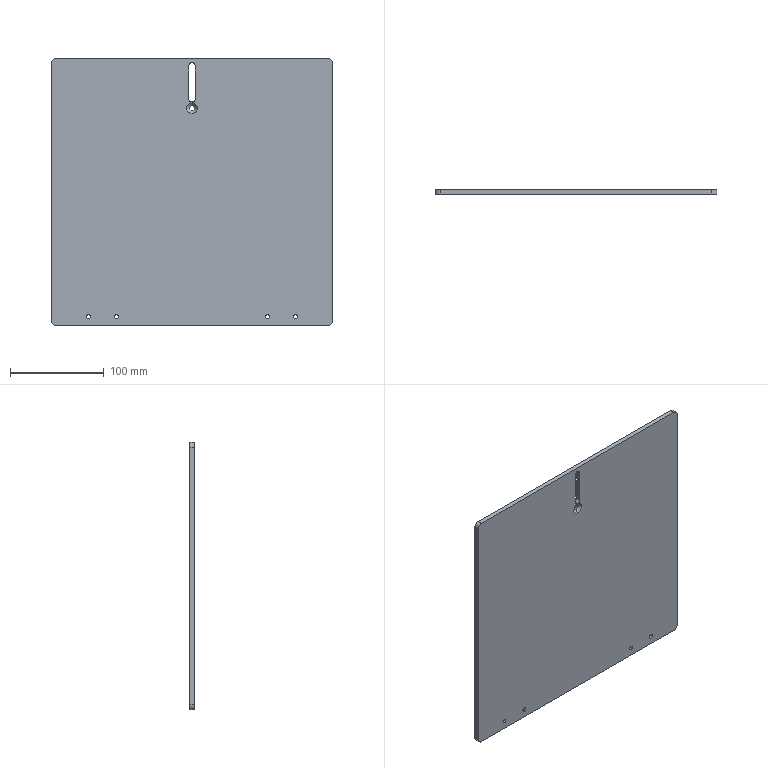Part | STEP file | ND22002-MA-D-007 | 1 solid | 27 faces | box 300 x 5 x 285 mm | volume 425473 mm3 | cylinder 17 | plane 8 | cone 2 | commonest cylinder face diameters 4.2 x8 10 x4 7 x3 5.5 x2